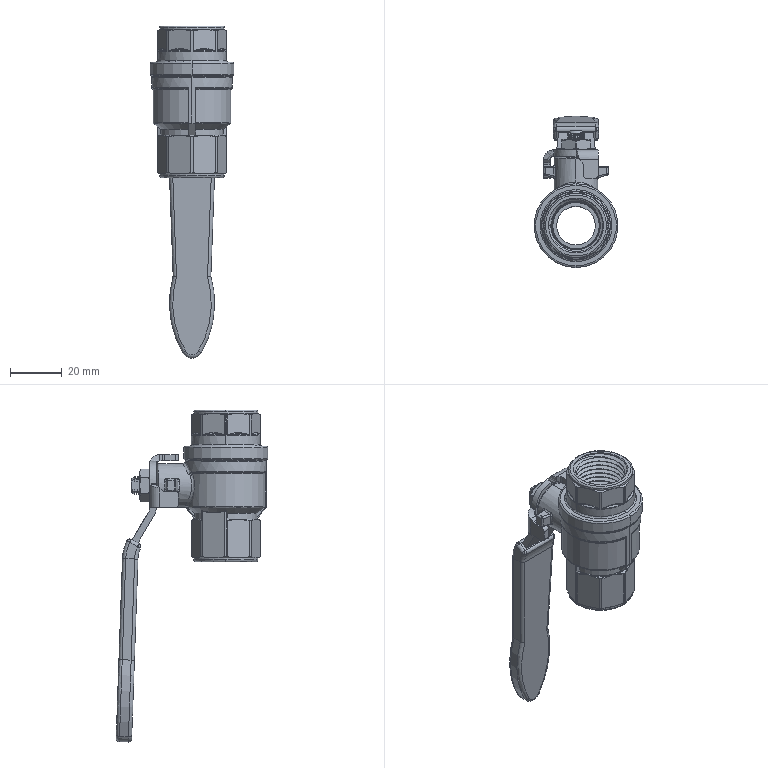Part | SolidWorks | 4 solids | 820 faces | box 32.512 x 58.766 x 128.692 mm | volume 33883 mm3 | spline 261 | plane 187 | cylinder 174 | cone 103 | sphere 52 | torus 43 | commonest cylinder face diameters 0.635 x62 7 x27 1.27 x20 2.54 x17 0.254 x6 24.221 x4